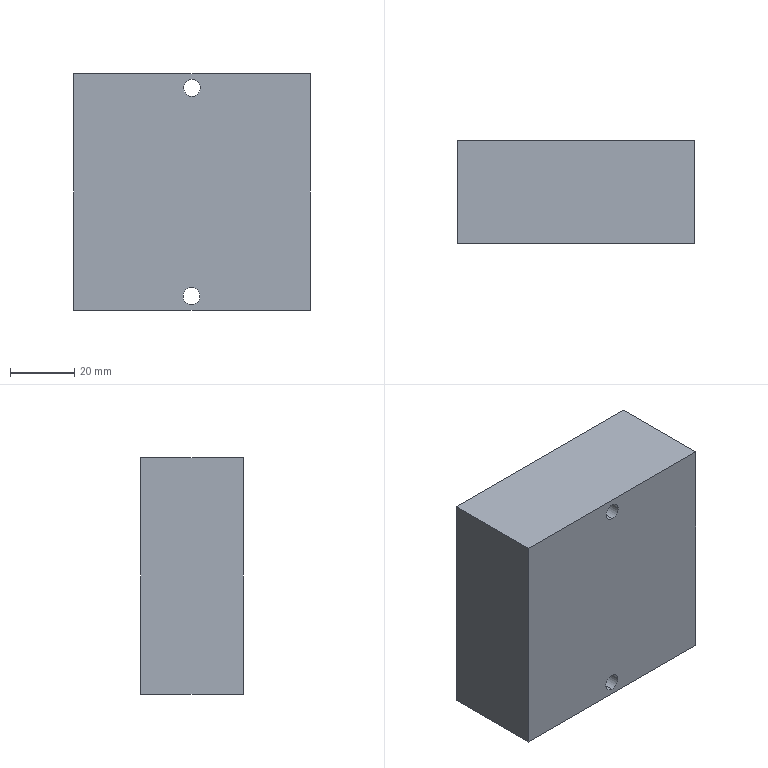Part | SolidWorks | features BaseBody 1 | 1 solid | 10 faces | box 74 x 32 x 74 mm | volume 173820 mm3 | plane 6 | cylinder 4 | commonest cylinder face diameters 5.3 x4
STEP:
#1=CARTESIAN_POINT('',(-4.95,140.,81.9));
#2=VERTEX_POINT('',#1);
#3=CARTESIAN_POINT('',(-4.95,140.,87.2));
#4=VERTEX_POINT('',#3);
#5=CARTESIAN_POINT('',(-4.95,140.,84.55));
#6=DIRECTION('',(0.,1.,0.));
#7=DIRECTION('',(0.,0.,-1.));
#8=AXIS2_PLACEMENT_3D('',#5,#6,#7);
#9=CIRCLE('',#8,2.65);
#10=EDGE_CURVE('',#2,#4,#9,.T.);
#11=ORIENTED_EDGE('',*,*,#10,.T.);
#12=CARTESIAN_POINT('',(-4.95,108.,87.2));
#13=VERTEX_POINT('',#12);
#14=CARTESIAN_POINT('',(-4.95,140.,87.2));
#15=DIRECTION('',(0.,-1.,0.));
#16=VECTOR('',#15,1000.);
#17=LINE('',#14,#16);
#18=EDGE_CURVE('',#4,#13,#17,.T.);
#19=ORIENTED_EDGE('',*,*,#18,.T.);
#20=CARTESIAN_POINT('',(-4.95,108.,81.9));
#21=VERTEX_POINT('',#20);
#22=CARTESIAN_POINT('',(-4.95,108.,84.55));
#23=DIRECTION('',(0.,1.,0.));
#24=DIRECTION('',(0.,0.,-1.));
#25=AXIS2_PLACEMENT_3D('',#22,#23,#24);
#26=CIRCLE('',#25,2.65);
#27=EDGE_CURVE('',#21,#13,#26,.T.);
#28=ORIENTED_EDGE('',*,*,#27,.F.);
#29=CARTESIAN_POINT('',(-4.95,140.,81.9));
#30=DIRECTION('',(0.,-1.,0.));
#31=VECTOR('',#30,1000.);
#32=LINE('',#29,#31);
#33=EDGE_CURVE('',#2,#21,#32,.T.);
#34=ORIENTED_EDGE('',*,*,#33,.F.);
#35=EDGE_LOOP('',(#11,#19,#28,#34));
#36=FACE_OUTER_BOUND('',#35,.T.);
#37=CARTESIAN_POINT('',(-4.95,140.,84.55));
#38=DIRECTION('',(0.,-1.,0.));
#39=DIRECTION('',(0.,0.,-1.));
#40=AXIS2_PLACEMENT_3D('',#37,#38,#39);
#41=CYLINDRICAL_SURFACE('',#40,2.65);
#42=ADVANCED_FACE('',(#36),#41,.F.);
#43=CARTESIAN_POINT('',(-5.1,140.,16.8));
#44=VERTEX_POINT('',#43);
#45=CARTESIAN_POINT('',(-5.1,140.,22.1));
#46=VERTEX_POINT('',#45);
#47=CARTESIAN_POINT('',(-5.1,140.,19.45));
#48=DIRECTION('',(0.,1.,0.));
#49=DIRECTION('',(0.,0.,-1.));
#50=AXIS2_PLACEMENT_3D('',#47,#48,#49);
#51=CIRCLE('',#50,2.65);
#52=EDGE_CURVE('',#44,#46,#51,.T.);
#53=ORIENTED_EDGE('',*,*,#52,.T.);
#54=CARTESIAN_POINT('',(-5.1,108.,22.1));
#55=VERTEX_POINT('',#54);
#56=CARTESIAN_POINT('',(-5.1,140.,22.1));
#57=DIRECTION('',(0.,-1.,0.));
#58=VECTOR('',#57,1000.);
#59=LINE('',#56,#58);
#60=EDGE_CURVE('',#46,#55,#59,.T.);
#61=ORIENTED_EDGE('',*,*,#60,.T.);
#62=CARTESIAN_POINT('',(-5.1,108.,16.8));
#63=VERTEX_POINT('',#62);
#64=CARTESIAN_POINT('',(-5.1,108.,19.45));
#65=DIRECTION('',(0.,1.,0.));
#66=DIRECTION('',(0.,0.,-1.));
#67=AXIS2_PLACEMENT_3D('',#64,#65,#66);
#68=CIRCLE('',#67,2.65);
#69=EDGE_CURVE('',#63,#55,#68,.T.);
#70=ORIENTED_EDGE('',*,*,#69,.F.);
#71=CARTESIAN_POINT('',(-5.1,140.,16.8));
#72=DIRECTION('',(0.,-1.,0.));
#73=VECTOR('',#72,1000.);
#74=LINE('',#71,#73);
#75=EDGE_CURVE('',#44,#63,#74,.T.);
#76=ORIENTED_EDGE('',*,*,#75,.F.);
#77=EDGE_LOOP('',(#53,#61,#70,#76));
#78=FACE_OUTER_BOUND('',#77,.T.);
#79=CARTESIAN_POINT('',(-5.1,140.,19.45));
#80=DIRECTION('',(0.,-1.,0.));
#81=DIRECTION('',(0.,0.,-1.));
#82=AXIS2_PLACEMENT_3D('',#79,#80,#81);
#83=CYLINDRICAL_SURFACE('',#82,2.65);
#84=ADVANCED_FACE('',(#78),#83,.F.);
#85=ORIENTED_EDGE('',*,*,#69,.T.);
#86=CARTESIAN_POINT('',(-5.1,108.,19.45));
#87=DIRECTION('',(0.,1.,0.));
#88=DIRECTION('',(0.,0.,-1.));
#89=AXIS2_PLACEMENT_3D('',#86,#87,#88);
#90=CIRCLE('',#89,2.65);
#91=EDGE_CURVE('',#55,#63,#90,.T.);
#92=ORIENTED_EDGE('',*,*,#91,.T.);
#93=EDGE_LOOP('',(#85,#92));
#94=FACE_BOUND('',#93,.T.);
#95=ORIENTED_EDGE('',*,*,#27,.T.);
#96=CARTESIAN_POINT('',(-4.95,108.,84.55));
#97=DIRECTION('',(0.,1.,0.));
#98=DIRECTION('',(0.,0.,-1.));
#99=AXIS2_PLACEMENT_3D('',#96,#97,#98);
#100=CIRCLE('',#99,2.65);
#101=EDGE_CURVE('',#13,#21,#100,.T.);
#102=ORIENTED_EDGE('',*,*,#101,.T.);
#103=EDGE_LOOP('',(#95,#102));
#104=FACE_BOUND('',#103,.T.);
#105=CARTESIAN_POINT('',(32.05,108.,15.));
#106=VERTEX_POINT('',#105);
#107=CARTESIAN_POINT('',(32.05,108.,89.));
#108=VERTEX_POINT('',#107);
#109=CARTESIAN_POINT('',(32.05,108.,89.));
#110=DIRECTION('',(0.,0.,1.));
#111=VECTOR('',#110,1000.);
#112=LINE('',#109,#111);
#113=EDGE_CURVE('',#106,#108,#112,.T.);
#114=ORIENTED_EDGE('',*,*,#113,.T.);
#115=CARTESIAN_POINT('',(-41.95,108.,89.));
#116=VERTEX_POINT('',#115);
#117=CARTESIAN_POINT('',(-41.95,108.,89.));
#118=DIRECTION('',(-1.,0.,0.));
#119=VECTOR('',#118,1000.);
#120=LINE('',#117,#119);
#121=EDGE_CURVE('',#108,#116,#120,.T.);
#122=ORIENTED_EDGE('',*,*,#121,.T.);
#123=CARTESIAN_POINT('',(-41.95,108.,15.));
#124=VERTEX_POINT('',#123);
#125=CARTESIAN_POINT('',(-41.95,108.,15.));
#126=DIRECTION('',(0.,0.,-1.));
#127=VECTOR('',#126,1000.);
#128=LINE('',#125,#127);
#129=EDGE_CURVE('',#116,#124,#128,.T.);
#130=ORIENTED_EDGE('',*,*,#129,.T.);
#131=CARTESIAN_POINT('',(32.05,108.,15.));
#132=DIRECTION('',(1.,0.,0.));
#133=VECTOR('',#132,1000.);
#134=LINE('',#131,#133);
#135=EDGE_CURVE('',#124,#106,#134,.T.);
#136=ORIENTED_EDGE('',*,*,#135,.T.);
#137=EDGE_LOOP('',(#114,#122,#130,#136));
#138=FACE_OUTER_BOUND('',#137,.T.);
#139=CARTESIAN_POINT('',(-4.95,108.,84.55));
#140=DIRECTION('',(0.,-1.,0.));
#141=DIRECTION('',(0.,0.,-1.));
#142=AXIS2_PLACEMENT_3D('',#139,#140,#141);
#143=PLANE('',#142);
#144=ADVANCED_FACE('',(#94,#104,#138),#143,.T.);
#145=CARTESIAN_POINT('',(32.05,140.,15.));
#146=VERTEX_POINT('',#145);
#147=CARTESIAN_POINT('',(32.05,140.,89.));
#148=VERTEX_POINT('',#147);
#149=CARTESIAN_POINT('',(32.05,140.,84.55));
#150=DIRECTION('',(0.,0.,1.));
#151=VECTOR('',#150,1000.);
#152=LINE('',#149,#151);
#153=EDGE_CURVE('',#146,#148,#152,.T.);
#154=ORIENTED_EDGE('',*,*,#153,.T.);
#155=CARTESIAN_POINT('',(32.05,140.,89.));
#156=DIRECTION('',(0.,-1.,0.));
#157=VECTOR('',#156,1000.);
#158=LINE('',#155,#157);
#159=EDGE_CURVE('',#148,#108,#158,.T.);
#160=ORIENTED_EDGE('',*,*,#159,.T.);
#161=ORIENTED_EDGE('',*,*,#113,.F.);
#162=CARTESIAN_POINT('',(32.05,140.,15.));
#163=DIRECTION('',(0.,1.,0.));
#164=VECTOR('',#163,1000.);
#165=LINE('',#162,#164);
#166=EDGE_CURVE('',#106,#146,#165,.T.);
#167=ORIENTED_EDGE('',*,*,#166,.T.);
#168=EDGE_LOOP('',(#154,#160,#161,#167));
#169=FACE_OUTER_BOUND('',#168,.T.);
#170=CARTESIAN_POINT('',(32.05,140.,89.));
#171=DIRECTION('',(-1.,0.,0.));
#172=DIRECTION('',(0.,0.,1.));
#173=AXIS2_PLACEMENT_3D('',#170,#171,#172);
#174=PLANE('',#173);
#175=ADVANCED_FACE('',(#169),#174,.F.);
#176=CARTESIAN_POINT('',(-41.95,140.,89.));
#177=VERTEX_POINT('',#176);
#178=CARTESIAN_POINT('',(-4.95,140.,89.));
#179=DIRECTION('',(-1.,0.,0.));
#180=VECTOR('',#179,1000.);
#181=LINE('',#178,#180);
#182=EDGE_CURVE('',#148,#177,#181,.T.);
#183=ORIENTED_EDGE('',*,*,#182,.T.);
#184=CARTESIAN_POINT('',(-41.95,140.,89.));
#185=DIRECTION('',(0.,-1.,0.));
#186=VECTOR('',#185,1000.);
#187=LINE('',#184,#186);
#188=EDGE_CURVE('',#177,#116,#187,.T.);
#189=ORIENTED_EDGE('',*,*,#188,.T.);
#190=ORIENTED_EDGE('',*,*,#121,.F.);
#191=ORIENTED_EDGE('',*,*,#159,.F.);
#192=EDGE_LOOP('',(#183,#189,#190,#191));
#193=FACE_OUTER_BOUND('',#192,.T.);
#194=CARTESIAN_POINT('',(-41.95,140.,89.));
#195=DIRECTION('',(0.,0.,-1.));
#196=DIRECTION('',(0.,-1.,0.));
#197=AXIS2_PLACEMENT_3D('',#194,#195,#196);
#198=PLANE('',#197);
#199=ADVANCED_FACE('',(#193),#198,.F.);
#200=CARTESIAN_POINT('',(-41.95,140.,15.));
#201=VERTEX_POINT('',#200);
#202=CARTESIAN_POINT('',(-41.95,140.,84.55));
#203=DIRECTION('',(0.,0.,-1.));
#204=VECTOR('',#203,1000.);
#205=LINE('',#202,#204);
#206=EDGE_CURVE('',#177,#201,#205,.T.);
#207=ORIENTED_EDGE('',*,*,#206,.T.);
#208=CARTESIAN_POINT('',(-41.95,140.,15.));
#209=DIRECTION('',(0.,-1.,0.));
#210=VECTOR('',#209,1000.);
#211=LINE('',#208,#210);
#212=EDGE_CURVE('',#201,#124,#211,.T.);
#213=ORIENTED_EDGE('',*,*,#212,.T.);
#214=ORIENTED_EDGE('',*,*,#129,.F.);
#215=ORIENTED_EDGE('',*,*,#188,.F.);
#216=EDGE_LOOP('',(#207,#213,#214,#215));
#217=FACE_OUTER_BOUND('',#216,.T.);
#218=CARTESIAN_POINT('',(-41.95,140.,15.));
#219=DIRECTION('',(1.,0.,0.));
#220=DIRECTION('',(0.,1.,0.));
#221=AXIS2_PLACEMENT_3D('',#218,#219,#220);
#222=PLANE('',#221);
#223=ADVANCED_FACE('',(#217),#222,.F.);
#224=CARTESIAN_POINT('',(-4.95,140.,15.));
#225=DIRECTION('',(1.,0.,0.));
#226=VECTOR('',#225,1000.);
#227=LINE('',#224,#226);
#228=EDGE_CURVE('',#201,#146,#227,.T.);
#229=ORIENTED_EDGE('',*,*,#228,.T.);
#230=ORIENTED_EDGE('',*,*,#166,.F.);
#231=ORIENTED_EDGE('',*,*,#135,.F.);
#232=ORIENTED_EDGE('',*,*,#212,.F.);
#233=EDGE_LOOP('',(#229,#230,#231,#232));
#234=FACE_OUTER_BOUND('',#233,.T.);
#235=CARTESIAN_POINT('',(32.05,140.,15.));
#236=DIRECTION('',(0.,0.,1.));
#237=DIRECTION('',(1.,0.,0.));
#238=AXIS2_PLACEMENT_3D('',#235,#236,#237);
#239=PLANE('',#238);
#240=ADVANCED_FACE('',(#234),#239,.F.);
#241=ORIENTED_EDGE('',*,*,#52,.F.);
#242=CARTESIAN_POINT('',(-5.1,140.,19.45));
#243=DIRECTION('',(0.,1.,0.));
#244=DIRECTION('',(0.,0.,-1.));
#245=AXIS2_PLACEMENT_3D('',#242,#243,#244);
#246=CIRCLE('',#245,2.65);
#247=EDGE_CURVE('',#46,#44,#246,.T.);
#248=ORIENTED_EDGE('',*,*,#247,.F.);
#249=EDGE_LOOP('',(#241,#248));
#250=FACE_BOUND('',#249,.T.);
#251=ORIENTED_EDGE('',*,*,#10,.F.);
#252=CARTESIAN_POINT('',(-4.95,140.,84.55));
#253=DIRECTION('',(0.,1.,0.));
#254=DIRECTION('',(0.,0.,-1.));
#255=AXIS2_PLACEMENT_3D('',#252,#253,#254);
#256=CIRCLE('',#255,2.65);
#257=EDGE_CURVE('',#4,#2,#256,.T.);
#258=ORIENTED_EDGE('',*,*,#257,.F.);
#259=EDGE_LOOP('',(#251,#258));
#260=FACE_BOUND('',#259,.T.);
#261=ORIENTED_EDGE('',*,*,#206,.F.);
#262=ORIENTED_EDGE('',*,*,#182,.F.);
#263=ORIENTED_EDGE('',*,*,#153,.F.);
#264=ORIENTED_EDGE('',*,*,#228,.F.);
#265=EDGE_LOOP('',(#261,#262,#263,#264));
#266=FACE_OUTER_BOUND('',#265,.T.);
#267=CARTESIAN_POINT('',(-4.95,140.,84.55));
#268=DIRECTION('',(0.,-1.,0.));
#269=DIRECTION('',(0.,0.,-1.));
#270=AXIS2_PLACEMENT_3D('',#267,#268,#269);
#271=PLANE('',#270);
#272=ADVANCED_FACE('',(#250,#260,#266),#271,.F.);
#273=ORIENTED_EDGE('',*,*,#60,.F.);
#274=ORIENTED_EDGE('',*,*,#247,.T.);
#275=ORIENTED_EDGE('',*,*,#75,.T.);
#276=ORIENTED_EDGE('',*,*,#91,.F.);
#277=EDGE_LOOP('',(#273,#274,#275,#276));
#278=FACE_OUTER_BOUND('',#277,.T.);
#279=CARTESIAN_POINT('',(-5.1,140.,19.45));
#280=DIRECTION('',(0.,-1.,0.));
#281=DIRECTION('',(0.,0.,-1.));
#282=AXIS2_PLACEMENT_3D('',#279,#280,#281);
#283=CYLINDRICAL_SURFACE('',#282,2.65);
#284=ADVANCED_FACE('',(#278),#283,.F.);
#285=ORIENTED_EDGE('',*,*,#18,.F.);
#286=ORIENTED_EDGE('',*,*,#257,.T.);
#287=ORIENTED_EDGE('',*,*,#33,.T.);
#288=ORIENTED_EDGE('',*,*,#101,.F.);
#289=EDGE_LOOP('',(#285,#286,#287,#288));
#290=FACE_OUTER_BOUND('',#289,.T.);
#291=CARTESIAN_POINT('',(-4.95,140.,84.55));
#292=DIRECTION('',(0.,-1.,0.));
#293=DIRECTION('',(0.,0.,-1.));
#294=AXIS2_PLACEMENT_3D('',#291,#292,#293);
#295=CYLINDRICAL_SURFACE('',#294,2.65);
#296=ADVANCED_FACE('',(#290),#295,.F.);
#297=CLOSED_SHELL('',(#42,#84,#144,#175,#199,#223,#240,#272,#284,#296));
#298=MANIFOLD_SOLID_BREP('',#297);
#299=CARTESIAN_POINT('',(0.,0.,0.));
#300=DIRECTION('',(0.,0.,1.));
#301=DIRECTION('',(1.,0.,0.));
#302=AXIS2_PLACEMENT_3D('',#299,#300,#301);
#303=(LENGTH_UNIT()NAMED_UNIT(*)SI_UNIT(.MILLI.,.METRE.));
#304=UNCERTAINTY_MEASURE_WITH_UNIT(LENGTH_MEASURE(0.00001),#303,'','');
#305=(NAMED_UNIT(*)PLANE_ANGLE_UNIT()SI_UNIT($,.RADIAN.));
#306=(NAMED_UNIT(*)SI_UNIT($,.STERADIAN.)SOLID_ANGLE_UNIT());
#307=(GEOMETRIC_REPRESENTATION_CONTEXT(3)GLOBAL_UNCERTAINTY_ASSIGNED_CONTEXT((#304))GLOBAL_UNIT_ASSIGNED_CONTEXT((#303,#305,#306))REPRESENTATION_CONTEXT('',''));
#308=ADVANCED_BREP_SHAPE_REPRESENTATION('',(#298,#302),#307);